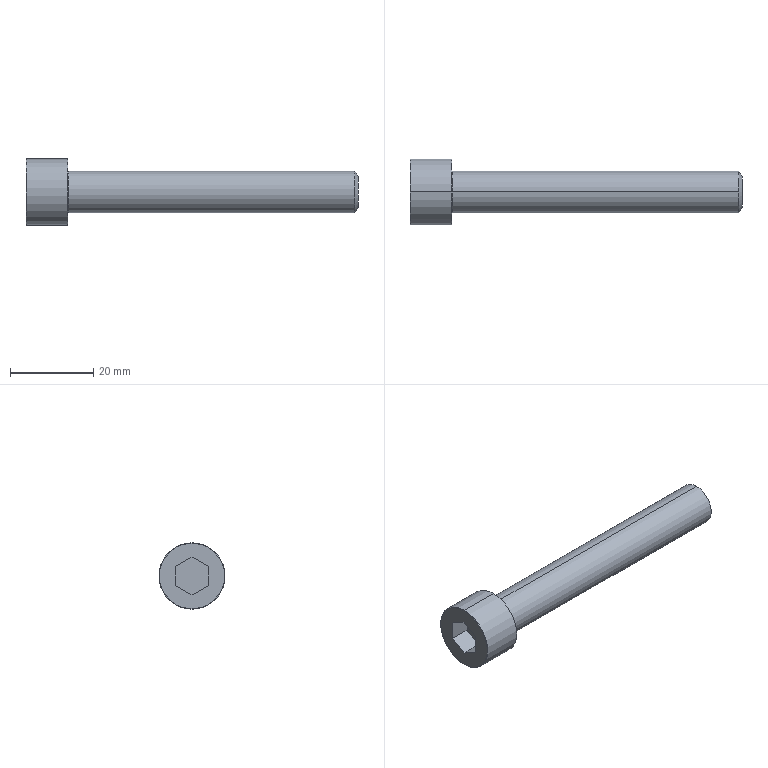Part | STEP file | 1 solid | 20 faces | box 80 x 16 x 16 mm | volume 7223 mm3 | plane 10 | torus 4 | cylinder 4 | cone 2 | commonest cylinder face diameters 10 x2 16 x2
STEP:
#1=CARTESIAN_POINT('',(0.,0.,7.9));
#2=VERTEX_POINT('',#1);
#3=CARTESIAN_POINT('',(0.,0.,-7.9));
#4=VERTEX_POINT('',#3);
#5=CARTESIAN_POINT('',(0.,0.,0.));
#6=DIRECTION('',(-1.,0.,0.));
#7=DIRECTION('',(0.,0.,-1.));
#8=AXIS2_PLACEMENT_3D('',#5,#6,#7);
#9=CIRCLE('',#8,7.9);
#10=EDGE_CURVE('',#2,#4,#9,.T.);
#11=ORIENTED_EDGE('',*,*,#10,.F.);
#12=CARTESIAN_POINT('',(0.1,0.,8.));
#13=VERTEX_POINT('',#12);
#14=CARTESIAN_POINT('',(0.1,0.,7.9));
#15=DIRECTION('',(0.,1.,0.));
#16=DIRECTION('',(0.,0.,1.));
#17=AXIS2_PLACEMENT_3D('',#14,#15,#16);
#18=CIRCLE('',#17,0.1);
#19=EDGE_CURVE('',#2,#13,#18,.T.);
#20=ORIENTED_EDGE('',*,*,#19,.T.);
#21=CARTESIAN_POINT('',(0.1,0.,-8.));
#22=VERTEX_POINT('',#21);
#23=CARTESIAN_POINT('',(0.1,0.,0.));
#24=DIRECTION('',(1.,0.,0.));
#25=DIRECTION('',(0.,0.,-1.));
#26=AXIS2_PLACEMENT_3D('',#23,#24,#25);
#27=CIRCLE('',#26,8.);
#28=EDGE_CURVE('',#22,#13,#27,.T.);
#29=ORIENTED_EDGE('',*,*,#28,.F.);
#30=CARTESIAN_POINT('',(0.1,0.,-7.9));
#31=DIRECTION('',(0.,-1.,0.));
#32=DIRECTION('',(0.,0.,-1.));
#33=AXIS2_PLACEMENT_3D('',#30,#31,#32);
#34=CIRCLE('',#33,0.1);
#35=EDGE_CURVE('',#4,#22,#34,.T.);
#36=ORIENTED_EDGE('',*,*,#35,.F.);
#37=EDGE_LOOP('',(#11,#20,#29,#36));
#38=FACE_OUTER_BOUND('',#37,.T.);
#39=CARTESIAN_POINT('',(0.1,0.,0.));
#40=DIRECTION('',(1.,0.,0.));
#41=DIRECTION('',(0.,0.,-1.));
#42=AXIS2_PLACEMENT_3D('',#39,#40,#41);
#43=TOROIDAL_SURFACE('',#42,7.9,0.1);
#44=ADVANCED_FACE('',(#38),#43,.T.);
#45=CARTESIAN_POINT('',(80.,0.,3.701));
#46=VERTEX_POINT('',#45);
#47=CARTESIAN_POINT('',(80.,0.,-3.701));
#48=VERTEX_POINT('',#47);
#49=CARTESIAN_POINT('',(80.,0.,0.));
#50=DIRECTION('',(-1.,0.,0.));
#51=DIRECTION('',(0.,0.,1.));
#52=AXIS2_PLACEMENT_3D('',#49,#50,#51);
#53=CIRCLE('',#52,3.701);
#54=EDGE_CURVE('',#46,#48,#53,.T.);
#55=ORIENTED_EDGE('',*,*,#54,.T.);
#56=CARTESIAN_POINT('',(79.25,0.,-5.));
#57=VERTEX_POINT('',#56);
#58=CARTESIAN_POINT('',(79.25,0.,-5.));
#59=DIRECTION('',(-0.5,0.,-0.866));
#60=VECTOR('',#59,1000.);
#61=LINE('',#58,#60);
#62=EDGE_CURVE('',#48,#57,#61,.T.);
#63=ORIENTED_EDGE('',*,*,#62,.T.);
#64=CARTESIAN_POINT('',(79.25,0.,5.));
#65=VERTEX_POINT('',#64);
#66=CARTESIAN_POINT('',(79.25,0.,0.));
#67=DIRECTION('',(-1.,0.,0.));
#68=DIRECTION('',(0.,0.,1.));
#69=AXIS2_PLACEMENT_3D('',#66,#67,#68);
#70=CIRCLE('',#69,5.);
#71=EDGE_CURVE('',#65,#57,#70,.T.);
#72=ORIENTED_EDGE('',*,*,#71,.F.);
#73=CARTESIAN_POINT('',(79.25,0.,5.));
#74=DIRECTION('',(-0.5,0.,0.866));
#75=VECTOR('',#74,1000.);
#76=LINE('',#73,#75);
#77=EDGE_CURVE('',#46,#65,#76,.T.);
#78=ORIENTED_EDGE('',*,*,#77,.F.);
#79=EDGE_LOOP('',(#55,#63,#72,#78));
#80=FACE_OUTER_BOUND('',#79,.T.);
#81=CARTESIAN_POINT('',(79.25,0.,0.));
#82=DIRECTION('',(-1.,0.,0.));
#83=DIRECTION('',(0.,0.,1.));
#84=AXIS2_PLACEMENT_3D('',#81,#82,#83);
#85=CONICAL_SURFACE('',#84,5.,1.047);
#86=ADVANCED_FACE('',(#80),#85,.T.);
#87=CARTESIAN_POINT('',(10.,0.,-5.2));
#88=VERTEX_POINT('',#87);
#89=CARTESIAN_POINT('',(10.,0.,5.2));
#90=VERTEX_POINT('',#89);
#91=CARTESIAN_POINT('',(10.,0.,0.));
#92=DIRECTION('',(-1.,0.,0.));
#93=DIRECTION('',(0.,0.,1.));
#94=AXIS2_PLACEMENT_3D('',#91,#92,#93);
#95=CIRCLE('',#94,5.2);
#96=EDGE_CURVE('',#88,#90,#95,.T.);
#97=ORIENTED_EDGE('',*,*,#96,.F.);
#98=CARTESIAN_POINT('',(10.2,0.,-5.));
#99=VERTEX_POINT('',#98);
#100=CARTESIAN_POINT('',(10.2,0.,-5.2));
#101=DIRECTION('',(0.,1.,0.));
#102=DIRECTION('',(0.,0.,1.));
#103=AXIS2_PLACEMENT_3D('',#100,#101,#102);
#104=CIRCLE('',#103,0.2);
#105=EDGE_CURVE('',#88,#99,#104,.T.);
#106=ORIENTED_EDGE('',*,*,#105,.T.);
#107=CARTESIAN_POINT('',(10.2,0.,5.));
#108=VERTEX_POINT('',#107);
#109=CARTESIAN_POINT('',(10.2,0.,0.));
#110=DIRECTION('',(-1.,0.,0.));
#111=DIRECTION('',(0.,0.,1.));
#112=AXIS2_PLACEMENT_3D('',#109,#110,#111);
#113=CIRCLE('',#112,5.);
#114=EDGE_CURVE('',#99,#108,#113,.T.);
#115=ORIENTED_EDGE('',*,*,#114,.T.);
#116=CARTESIAN_POINT('',(10.2,0.,5.2));
#117=DIRECTION('',(0.,-1.,0.));
#118=DIRECTION('',(0.,0.,-1.));
#119=AXIS2_PLACEMENT_3D('',#116,#117,#118);
#120=CIRCLE('',#119,0.2);
#121=EDGE_CURVE('',#90,#108,#120,.T.);
#122=ORIENTED_EDGE('',*,*,#121,.F.);
#123=EDGE_LOOP('',(#97,#106,#115,#122));
#124=FACE_OUTER_BOUND('',#123,.T.);
#125=CARTESIAN_POINT('',(10.2,0.,0.));
#126=DIRECTION('',(-1.,0.,0.));
#127=DIRECTION('',(0.,0.,1.));
#128=AXIS2_PLACEMENT_3D('',#125,#126,#127);
#129=TOROIDAL_SURFACE('',#128,5.2,0.2);
#130=ADVANCED_FACE('',(#124),#129,.F.);
#131=CARTESIAN_POINT('',(10.,0.,8.));
#132=VERTEX_POINT('',#131);
#133=CARTESIAN_POINT('',(10.,0.,-8.));
#134=VERTEX_POINT('',#133);
#135=CARTESIAN_POINT('',(10.,0.,0.));
#136=DIRECTION('',(-1.,0.,0.));
#137=DIRECTION('',(0.,0.,1.));
#138=AXIS2_PLACEMENT_3D('',#135,#136,#137);
#139=CIRCLE('',#138,8.);
#140=EDGE_CURVE('',#132,#134,#139,.T.);
#141=ORIENTED_EDGE('',*,*,#140,.T.);
#142=CARTESIAN_POINT('',(0.,0.,-8.));
#143=DIRECTION('',(-1.,0.,0.));
#144=VECTOR('',#143,1000.);
#145=LINE('',#142,#144);
#146=EDGE_CURVE('',#134,#22,#145,.T.);
#147=ORIENTED_EDGE('',*,*,#146,.T.);
#148=ORIENTED_EDGE('',*,*,#28,.T.);
#149=CARTESIAN_POINT('',(0.,0.,8.));
#150=DIRECTION('',(-1.,0.,0.));
#151=VECTOR('',#150,1000.);
#152=LINE('',#149,#151);
#153=EDGE_CURVE('',#132,#13,#152,.T.);
#154=ORIENTED_EDGE('',*,*,#153,.F.);
#155=EDGE_LOOP('',(#141,#147,#148,#154));
#156=FACE_OUTER_BOUND('',#155,.T.);
#157=CARTESIAN_POINT('',(0.,0.,0.));
#158=DIRECTION('',(-1.,0.,0.));
#159=DIRECTION('',(0.,0.,1.));
#160=AXIS2_PLACEMENT_3D('',#157,#158,#159);
#161=CYLINDRICAL_SURFACE('',#160,8.);
#162=ADVANCED_FACE('',(#156),#161,.T.);
#163=ORIENTED_EDGE('',*,*,#71,.T.);
#164=CARTESIAN_POINT('',(0.,0.,-5.));
#165=DIRECTION('',(-1.,0.,0.));
#166=VECTOR('',#165,1000.);
#167=LINE('',#164,#166);
#168=EDGE_CURVE('',#57,#99,#167,.T.);
#169=ORIENTED_EDGE('',*,*,#168,.T.);
#170=CARTESIAN_POINT('',(10.2,0.,0.));
#171=DIRECTION('',(-1.,0.,0.));
#172=DIRECTION('',(0.,0.,1.));
#173=AXIS2_PLACEMENT_3D('',#170,#171,#172);
#174=CIRCLE('',#173,5.);
#175=EDGE_CURVE('',#108,#99,#174,.T.);
#176=ORIENTED_EDGE('',*,*,#175,.F.);
#177=CARTESIAN_POINT('',(0.,0.,5.));
#178=DIRECTION('',(-1.,0.,0.));
#179=VECTOR('',#178,1000.);
#180=LINE('',#177,#179);
#181=EDGE_CURVE('',#65,#108,#180,.T.);
#182=ORIENTED_EDGE('',*,*,#181,.F.);
#183=EDGE_LOOP('',(#163,#169,#176,#182));
#184=FACE_OUTER_BOUND('',#183,.T.);
#185=CARTESIAN_POINT('',(0.,0.,0.));
#186=DIRECTION('',(-1.,0.,0.));
#187=DIRECTION('',(0.,0.,1.));
#188=AXIS2_PLACEMENT_3D('',#185,#186,#187);
#189=CYLINDRICAL_SURFACE('',#188,5.);
#190=ADVANCED_FACE('',(#184),#189,.T.);
#191=ORIENTED_EDGE('',*,*,#168,.F.);
#192=CARTESIAN_POINT('',(79.25,0.,0.));
#193=DIRECTION('',(-1.,0.,0.));
#194=DIRECTION('',(0.,0.,1.));
#195=AXIS2_PLACEMENT_3D('',#192,#193,#194);
#196=CIRCLE('',#195,5.);
#197=EDGE_CURVE('',#57,#65,#196,.T.);
#198=ORIENTED_EDGE('',*,*,#197,.T.);
#199=ORIENTED_EDGE('',*,*,#181,.T.);
#200=ORIENTED_EDGE('',*,*,#114,.F.);
#201=EDGE_LOOP('',(#191,#198,#199,#200));
#202=FACE_OUTER_BOUND('',#201,.T.);
#203=CARTESIAN_POINT('',(0.,0.,0.));
#204=DIRECTION('',(-1.,0.,0.));
#205=DIRECTION('',(0.,0.,1.));
#206=AXIS2_PLACEMENT_3D('',#203,#204,#205);
#207=CYLINDRICAL_SURFACE('',#206,5.);
#208=ADVANCED_FACE('',(#202),#207,.T.);
#209=CARTESIAN_POINT('',(0.,0.,0.));
#210=DIRECTION('',(-1.,0.,0.));
#211=DIRECTION('',(0.,0.,-1.));
#212=AXIS2_PLACEMENT_3D('',#209,#210,#211);
#213=CIRCLE('',#212,7.9);
#214=EDGE_CURVE('',#4,#2,#213,.T.);
#215=ORIENTED_EDGE('',*,*,#214,.T.);
#216=ORIENTED_EDGE('',*,*,#10,.T.);
#217=EDGE_LOOP('',(#215,#216));
#218=FACE_OUTER_BOUND('',#217,.T.);
#219=CARTESIAN_POINT('',(0.,0.,4.575));
#220=VERTEX_POINT('',#219);
#221=CARTESIAN_POINT('',(0.,3.962,2.287));
#222=VERTEX_POINT('',#221);
#223=CARTESIAN_POINT('',(0.,0.,4.575));
#224=DIRECTION('',(0.,0.866,-0.5));
#225=VECTOR('',#224,1000.);
#226=LINE('',#223,#225);
#227=EDGE_CURVE('',#220,#222,#226,.T.);
#228=ORIENTED_EDGE('',*,*,#227,.F.);
#229=CARTESIAN_POINT('',(0.,-3.962,2.288));
#230=VERTEX_POINT('',#229);
#231=CARTESIAN_POINT('',(0.,-3.962,2.288));
#232=DIRECTION('',(0.,0.866,0.5));
#233=VECTOR('',#232,1000.);
#234=LINE('',#231,#233);
#235=EDGE_CURVE('',#230,#220,#234,.T.);
#236=ORIENTED_EDGE('',*,*,#235,.F.);
#237=CARTESIAN_POINT('',(0.,-3.962,-2.288));
#238=VERTEX_POINT('',#237);
#239=CARTESIAN_POINT('',(0.,-3.962,-2.288));
#240=DIRECTION('',(0.,0.,1.));
#241=VECTOR('',#240,1000.);
#242=LINE('',#239,#241);
#243=EDGE_CURVE('',#238,#230,#242,.T.);
#244=ORIENTED_EDGE('',*,*,#243,.F.);
#245=CARTESIAN_POINT('',(0.,0.,-4.575));
#246=VERTEX_POINT('',#245);
#247=CARTESIAN_POINT('',(0.,0.,-4.575));
#248=DIRECTION('',(0.,-0.866,0.5));
#249=VECTOR('',#248,1000.);
#250=LINE('',#247,#249);
#251=EDGE_CURVE('',#246,#238,#250,.T.);
#252=ORIENTED_EDGE('',*,*,#251,.F.);
#253=CARTESIAN_POINT('',(0.,3.962,-2.287));
#254=VERTEX_POINT('',#253);
#255=CARTESIAN_POINT('',(0.,3.962,-2.287));
#256=DIRECTION('',(0.,-0.866,-0.5));
#257=VECTOR('',#256,1000.);
#258=LINE('',#255,#257);
#259=EDGE_CURVE('',#254,#246,#258,.T.);
#260=ORIENTED_EDGE('',*,*,#259,.F.);
#261=CARTESIAN_POINT('',(0.,3.962,2.287));
#262=DIRECTION('',(0.,0.,-1.));
#263=VECTOR('',#262,1000.);
#264=LINE('',#261,#263);
#265=EDGE_CURVE('',#222,#254,#264,.T.);
#266=ORIENTED_EDGE('',*,*,#265,.F.);
#267=EDGE_LOOP('',(#228,#236,#244,#252,#260,#266));
#268=FACE_BOUND('',#267,.T.);
#269=CARTESIAN_POINT('',(0.,0.,0.));
#270=DIRECTION('',(1.,0.,0.));
#271=DIRECTION('',(0.,0.,-1.));
#272=AXIS2_PLACEMENT_3D('',#269,#270,#271);
#273=PLANE('',#272);
#274=ADVANCED_FACE('',(#218,#268),#273,.F.);
#275=ORIENTED_EDGE('',*,*,#146,.F.);
#276=CARTESIAN_POINT('',(10.,0.,0.));
#277=DIRECTION('',(-1.,0.,0.));
#278=DIRECTION('',(0.,0.,1.));
#279=AXIS2_PLACEMENT_3D('',#276,#277,#278);
#280=CIRCLE('',#279,8.);
#281=EDGE_CURVE('',#134,#132,#280,.T.);
#282=ORIENTED_EDGE('',*,*,#281,.T.);
#283=ORIENTED_EDGE('',*,*,#153,.T.);
#284=CARTESIAN_POINT('',(0.1,0.,0.));
#285=DIRECTION('',(1.,0.,0.));
#286=DIRECTION('',(0.,0.,-1.));
#287=AXIS2_PLACEMENT_3D('',#284,#285,#286);
#288=CIRCLE('',#287,8.);
#289=EDGE_CURVE('',#13,#22,#288,.T.);
#290=ORIENTED_EDGE('',*,*,#289,.T.);
#291=EDGE_LOOP('',(#275,#282,#283,#290));
#292=FACE_OUTER_BOUND('',#291,.T.);
#293=CARTESIAN_POINT('',(0.,0.,0.));
#294=DIRECTION('',(-1.,0.,0.));
#295=DIRECTION('',(0.,0.,1.));
#296=AXIS2_PLACEMENT_3D('',#293,#294,#295);
#297=CYLINDRICAL_SURFACE('',#296,8.);
#298=ADVANCED_FACE('',(#292),#297,.T.);
#299=ORIENTED_EDGE('',*,*,#140,.F.);
#300=ORIENTED_EDGE('',*,*,#281,.F.);
#301=EDGE_LOOP('',(#299,#300));
#302=FACE_OUTER_BOUND('',#301,.T.);
#303=CARTESIAN_POINT('',(10.,0.,0.));
#304=DIRECTION('',(-1.,0.,0.));
#305=DIRECTION('',(0.,0.,1.));
#306=AXIS2_PLACEMENT_3D('',#303,#304,#305);
#307=CIRCLE('',#306,5.2);
#308=EDGE_CURVE('',#90,#88,#307,.T.);
#309=ORIENTED_EDGE('',*,*,#308,.T.);
#310=ORIENTED_EDGE('',*,*,#96,.T.);
#311=EDGE_LOOP('',(#309,#310));
#312=FACE_BOUND('',#311,.T.);
#313=CARTESIAN_POINT('',(10.,8.,0.));
#314=DIRECTION('',(-1.,0.,0.));
#315=DIRECTION('',(0.,0.,1.));
#316=AXIS2_PLACEMENT_3D('',#313,#314,#315);
#317=PLANE('',#316);
#318=ADVANCED_FACE('',(#302,#312),#317,.F.);
#319=ORIENTED_EDGE('',*,*,#105,.F.);
#320=ORIENTED_EDGE('',*,*,#308,.F.);
#321=ORIENTED_EDGE('',*,*,#121,.T.);
#322=ORIENTED_EDGE('',*,*,#175,.T.);
#323=EDGE_LOOP('',(#319,#320,#321,#322));
#324=FACE_OUTER_BOUND('',#323,.T.);
#325=CARTESIAN_POINT('',(10.2,0.,0.));
#326=DIRECTION('',(-1.,0.,0.));
#327=DIRECTION('',(0.,0.,1.));
#328=AXIS2_PLACEMENT_3D('',#325,#326,#327);
#329=TOROIDAL_SURFACE('',#328,5.2,0.2);
#330=ADVANCED_FACE('',(#324),#329,.F.);
#331=ORIENTED_EDGE('',*,*,#235,.T.);
#332=CARTESIAN_POINT('',(5.,0.,4.575));
#333=VERTEX_POINT('',#332);
#334=CARTESIAN_POINT('',(5.,0.,4.575));
#335=DIRECTION('',(-1.,0.,0.));
#336=VECTOR('',#335,1000.);
#337=LINE('',#334,#336);
#338=EDGE_CURVE('',#333,#220,#337,.T.);
#339=ORIENTED_EDGE('',*,*,#338,.F.);
#340=CARTESIAN_POINT('',(5.,-3.962,2.288));
#341=VERTEX_POINT('',#340);
#342=CARTESIAN_POINT('',(5.,-3.962,2.288));
#343=DIRECTION('',(0.,0.866,0.5));
#344=VECTOR('',#343,1000.);
#345=LINE('',#342,#344);
#346=EDGE_CURVE('',#341,#333,#345,.T.);
#347=ORIENTED_EDGE('',*,*,#346,.F.);
#348=CARTESIAN_POINT('',(5.,-3.962,2.288));
#349=DIRECTION('',(-1.,0.,0.));
#350=VECTOR('',#349,1000.);
#351=LINE('',#348,#350);
#352=EDGE_CURVE('',#341,#230,#351,.T.);
#353=ORIENTED_EDGE('',*,*,#352,.T.);
#354=EDGE_LOOP('',(#331,#339,#347,#353));
#355=FACE_OUTER_BOUND('',#354,.T.);
#356=CARTESIAN_POINT('',(5.,-3.962,2.288));
#357=DIRECTION('',(0.,-0.5,0.866));
#358=DIRECTION('',(0.,-0.866,-0.5));
#359=AXIS2_PLACEMENT_3D('',#356,#357,#358);
#360=PLANE('',#359);
#361=ADVANCED_FACE('',(#355),#360,.F.);
#362=ORIENTED_EDGE('',*,*,#243,.T.);
#363=ORIENTED_EDGE('',*,*,#352,.F.);
#364=CARTESIAN_POINT('',(5.,-3.962,-2.288));
#365=VERTEX_POINT('',#364);
#366=CARTESIAN_POINT('',(5.,-3.962,-2.288));
#367=DIRECTION('',(0.,0.,1.));
#368=VECTOR('',#367,1000.);
#369=LINE('',#366,#368);
#370=EDGE_CURVE('',#365,#341,#369,.T.);
#371=ORIENTED_EDGE('',*,*,#370,.F.);
#372=CARTESIAN_POINT('',(5.,-3.962,-2.288));
#373=DIRECTION('',(-1.,0.,0.));
#374=VECTOR('',#373,1000.);
#375=LINE('',#372,#374);
#376=EDGE_CURVE('',#365,#238,#375,.T.);
#377=ORIENTED_EDGE('',*,*,#376,.T.);
#378=EDGE_LOOP('',(#362,#363,#371,#377));
#379=FACE_OUTER_BOUND('',#378,.T.);
#380=CARTESIAN_POINT('',(5.,-3.962,-2.288));
#381=DIRECTION('',(0.,-1.,0.));
#382=DIRECTION('',(0.,0.,-1.));
#383=AXIS2_PLACEMENT_3D('',#380,#381,#382);
#384=PLANE('',#383);
#385=ADVANCED_FACE('',(#379),#384,.F.);
#386=ORIENTED_EDGE('',*,*,#251,.T.);
#387=ORIENTED_EDGE('',*,*,#376,.F.);
#388=CARTESIAN_POINT('',(5.,0.,-4.575));
#389=VERTEX_POINT('',#388);
#390=CARTESIAN_POINT('',(5.,0.,-4.575));
#391=DIRECTION('',(0.,-0.866,0.5));
#392=VECTOR('',#391,1000.);
#393=LINE('',#390,#392);
#394=EDGE_CURVE('',#389,#365,#393,.T.);
#395=ORIENTED_EDGE('',*,*,#394,.F.);
#396=CARTESIAN_POINT('',(5.,0.,-4.575));
#397=DIRECTION('',(-1.,0.,0.));
#398=VECTOR('',#397,1000.);
#399=LINE('',#396,#398);
#400=EDGE_CURVE('',#389,#246,#399,.T.);
#401=ORIENTED_EDGE('',*,*,#400,.T.);
#402=EDGE_LOOP('',(#386,#387,#395,#401));
#403=FACE_OUTER_BOUND('',#402,.T.);
#404=CARTESIAN_POINT('',(5.,0.,-4.575));
#405=DIRECTION('',(0.,-0.5,-0.866));
#406=DIRECTION('',(0.,0.866,-0.5));
#407=AXIS2_PLACEMENT_3D('',#404,#405,#406);
#408=PLANE('',#407);
#409=ADVANCED_FACE('',(#403),#408,.F.);
#410=ORIENTED_EDGE('',*,*,#259,.T.);
#411=ORIENTED_EDGE('',*,*,#400,.F.);
#412=CARTESIAN_POINT('',(5.,3.962,-2.287));
#413=VERTEX_POINT('',#412);
#414=CARTESIAN_POINT('',(5.,3.962,-2.287));
#415=DIRECTION('',(0.,-0.866,-0.5));
#416=VECTOR('',#415,1000.);
#417=LINE('',#414,#416);
#418=EDGE_CURVE('',#413,#389,#417,.T.);
#419=ORIENTED_EDGE('',*,*,#418,.F.);
#420=CARTESIAN_POINT('',(5.,3.962,-2.287));
#421=DIRECTION('',(-1.,0.,0.));
#422=VECTOR('',#421,1000.);
#423=LINE('',#420,#422);
#424=EDGE_CURVE('',#413,#254,#423,.T.);
#425=ORIENTED_EDGE('',*,*,#424,.T.);
#426=EDGE_LOOP('',(#410,#411,#419,#425));
#427=FACE_OUTER_BOUND('',#426,.T.);
#428=CARTESIAN_POINT('',(5.,3.962,-2.287));
#429=DIRECTION('',(0.,0.5,-0.866));
#430=DIRECTION('',(0.,0.866,0.5));
#431=AXIS2_PLACEMENT_3D('',#428,#429,#430);
#432=PLANE('',#431);
#433=ADVANCED_FACE('',(#427),#432,.F.);
#434=ORIENTED_EDGE('',*,*,#265,.T.);
#435=ORIENTED_EDGE('',*,*,#424,.F.);
#436=CARTESIAN_POINT('',(5.,3.962,2.287));
#437=VERTEX_POINT('',#436);
#438=CARTESIAN_POINT('',(5.,3.962,2.287));
#439=DIRECTION('',(0.,0.,-1.));
#440=VECTOR('',#439,1000.);
#441=LINE('',#438,#440);
#442=EDGE_CURVE('',#437,#413,#441,.T.);
#443=ORIENTED_EDGE('',*,*,#442,.F.);
#444=CARTESIAN_POINT('',(5.,3.962,2.287));
#445=DIRECTION('',(-1.,0.,0.));
#446=VECTOR('',#445,1000.);
#447=LINE('',#444,#446);
#448=EDGE_CURVE('',#437,#222,#447,.T.);
#449=ORIENTED_EDGE('',*,*,#448,.T.);
#450=EDGE_LOOP('',(#434,#435,#443,#449));
#451=FACE_OUTER_BOUND('',#450,.T.);
#452=CARTESIAN_POINT('',(5.,3.962,2.287));
#453=DIRECTION('',(0.,1.,0.));
#454=DIRECTION('',(0.,0.,1.));
#455=AXIS2_PLACEMENT_3D('',#452,#453,#454);
#456=PLANE('',#455);
#457=ADVANCED_FACE('',(#451),#456,.F.);
#458=ORIENTED_EDGE('',*,*,#227,.T.);
#459=ORIENTED_EDGE('',*,*,#448,.F.);
#460=CARTESIAN_POINT('',(5.,0.,4.575));
#461=DIRECTION('',(0.,0.866,-0.5));
#462=VECTOR('',#461,1000.);
#463=LINE('',#460,#462);
#464=EDGE_CURVE('',#333,#437,#463,.T.);
#465=ORIENTED_EDGE('',*,*,#464,.F.);
#466=ORIENTED_EDGE('',*,*,#338,.T.);
#467=EDGE_LOOP('',(#458,#459,#465,#466));
#468=FACE_OUTER_BOUND('',#467,.T.);
#469=CARTESIAN_POINT('',(5.,0.,4.575));
#470=DIRECTION('',(0.,0.5,0.866));
#471=DIRECTION('',(0.,-0.866,0.5));
#472=AXIS2_PLACEMENT_3D('',#469,#470,#471);
#473=PLANE('',#472);
#474=ADVANCED_FACE('',(#468),#473,.F.);
#475=ORIENTED_EDGE('',*,*,#346,.T.);
#476=ORIENTED_EDGE('',*,*,#464,.T.);
#477=ORIENTED_EDGE('',*,*,#442,.T.);
#478=ORIENTED_EDGE('',*,*,#418,.T.);
#479=ORIENTED_EDGE('',*,*,#394,.T.);
#480=ORIENTED_EDGE('',*,*,#370,.T.);
#481=EDGE_LOOP('',(#475,#476,#477,#478,#479,#480));
#482=FACE_OUTER_BOUND('',#481,.T.);
#483=CARTESIAN_POINT('',(5.,-3.962,2.288));
#484=DIRECTION('',(1.,0.,0.));
#485=DIRECTION('',(0.,0.,-1.));
#486=AXIS2_PLACEMENT_3D('',#483,#484,#485);
#487=PLANE('',#486);
#488=ADVANCED_FACE('',(#482),#487,.F.);
#489=ORIENTED_EDGE('',*,*,#62,.F.);
#490=CARTESIAN_POINT('',(80.,0.,0.));
#491=DIRECTION('',(-1.,0.,0.));
#492=DIRECTION('',(0.,0.,1.));
#493=AXIS2_PLACEMENT_3D('',#490,#491,#492);
#494=CIRCLE('',#493,3.701);
#495=EDGE_CURVE('',#48,#46,#494,.T.);
#496=ORIENTED_EDGE('',*,*,#495,.T.);
#497=ORIENTED_EDGE('',*,*,#77,.T.);
#498=ORIENTED_EDGE('',*,*,#197,.F.);
#499=EDGE_LOOP('',(#489,#496,#497,#498));
#500=FACE_OUTER_BOUND('',#499,.T.);
#501=CARTESIAN_POINT('',(79.25,0.,0.));
#502=DIRECTION('',(-1.,0.,0.));
#503=DIRECTION('',(0.,0.,1.));
#504=AXIS2_PLACEMENT_3D('',#501,#502,#503);
#505=CONICAL_SURFACE('',#504,5.,1.047);
#506=ADVANCED_FACE('',(#500),#505,.T.);
#507=ORIENTED_EDGE('',*,*,#54,.F.);
#508=ORIENTED_EDGE('',*,*,#495,.F.);
#509=EDGE_LOOP('',(#507,#508));
#510=FACE_OUTER_BOUND('',#509,.T.);
#511=CARTESIAN_POINT('',(80.,5.,0.));
#512=DIRECTION('',(-1.,0.,0.));
#513=DIRECTION('',(0.,0.,1.));
#514=AXIS2_PLACEMENT_3D('',#511,#512,#513);
#515=PLANE('',#514);
#516=ADVANCED_FACE('',(#510),#515,.F.);
#517=ORIENTED_EDGE('',*,*,#19,.F.);
#518=ORIENTED_EDGE('',*,*,#214,.F.);
#519=ORIENTED_EDGE('',*,*,#35,.T.);
#520=ORIENTED_EDGE('',*,*,#289,.F.);
#521=EDGE_LOOP('',(#517,#518,#519,#520));
#522=FACE_OUTER_BOUND('',#521,.T.);
#523=CARTESIAN_POINT('',(0.1,0.,0.));
#524=DIRECTION('',(1.,0.,0.));
#525=DIRECTION('',(0.,0.,-1.));
#526=AXIS2_PLACEMENT_3D('',#523,#524,#525);
#527=TOROIDAL_SURFACE('',#526,7.9,0.1);
#528=ADVANCED_FACE('',(#522),#527,.T.);
#529=CLOSED_SHELL('',(#44,#86,#130,#162,#190,#208,#274,#298,#318,#330,#361,#385,#409,#433,#457,#474,#488,#506,#516,#528));
#530=MANIFOLD_SOLID_BREP('',#529);
#531=CARTESIAN_POINT('',(0.,0.,0.));
#532=DIRECTION('',(0.,0.,1.));
#533=DIRECTION('',(1.,0.,0.));
#534=AXIS2_PLACEMENT_3D('',#531,#532,#533);
#535=(LENGTH_UNIT()NAMED_UNIT(*)SI_UNIT(.MILLI.,.METRE.));
#536=UNCERTAINTY_MEASURE_WITH_UNIT(LENGTH_MEASURE(0.00001),#535,'','');
#537=(NAMED_UNIT(*)PLANE_ANGLE_UNIT()SI_UNIT($,.RADIAN.));
#538=(NAMED_UNIT(*)SI_UNIT($,.STERADIAN.)SOLID_ANGLE_UNIT());
#539=(GEOMETRIC_REPRESENTATION_CONTEXT(3)GLOBAL_UNCERTAINTY_ASSIGNED_CONTEXT((#536))GLOBAL_UNIT_ASSIGNED_CONTEXT((#535,#537,#538))REPRESENTATION_CONTEXT('',''));
#540=ADVANCED_BREP_SHAPE_REPRESENTATION('',(#530,#534),#539);